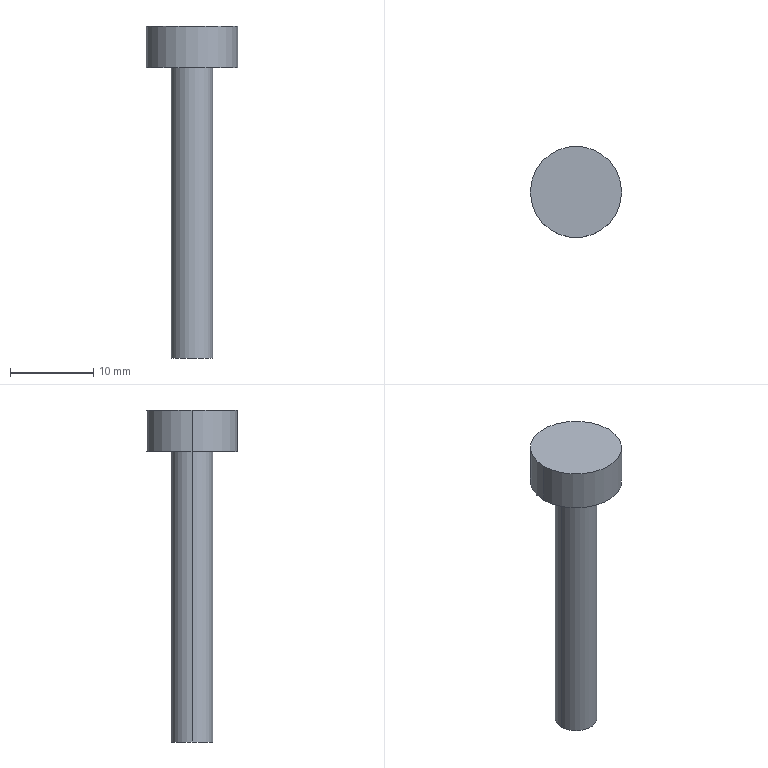Part | STEP file | Pull rod | 1 solid | 7 faces | box 11 x 11 x 40 mm | volume 1162 mm3 | cylinder 4 | plane 3 | commonest cylinder face diameters 5 x2 11 x2
STEP:
#1=CARTESIAN_POINT('',(0.,0.,0.));
#2=DIRECTION('',(0.,0.,1.));
#3=DIRECTION('',(1.,0.,0.));
#4=AXIS2_PLACEMENT_3D('',#1,#2,#3);
#5=CARTESIAN_POINT('',(-2.5,0.,-35.));
#6=VERTEX_POINT('',#5);
#7=CARTESIAN_POINT('',(2.5,0.,-35.));
#8=VERTEX_POINT('',#7);
#9=CARTESIAN_POINT('',(0.,0.,-35.));
#10=DIRECTION('',(0.,0.,-1.));
#11=DIRECTION('',(-1.,0.,0.));
#12=AXIS2_PLACEMENT_3D('',#9,#10,#11);
#13=CIRCLE('',#12,2.5);
#14=CARTESIAN_POINT('',(0.,0.,-35.));
#15=DIRECTION('',(0.,0.,1.));
#16=DIRECTION('',(1.,0.,0.));
#17=AXIS2_PLACEMENT_3D('',#14,#15,#16);
#18=CYLINDRICAL_SURFACE('',#17,2.5);
#19=CARTESIAN_POINT('',(3.142,0.));
#20=DIRECTION('',(-1.,0.));
#21=VECTOR('',#20,1.);
#22=LINE('',#19,#21);
#23=(GEOMETRIC_REPRESENTATION_CONTEXT(2)PARAMETRIC_REPRESENTATION_CONTEXT()REPRESENTATION_CONTEXT('',''));
#24=DEFINITIONAL_REPRESENTATION('',(#22),#23);
#25=PCURVE('',#18,#24);
#26=CARTESIAN_POINT('',(0.,0.,-35.));
#27=DIRECTION('',(0.,0.,-1.));
#28=DIRECTION('',(-1.,0.,0.));
#29=AXIS2_PLACEMENT_3D('',#26,#27,#28);
#30=PLANE('',#29);
#31=CARTESIAN_POINT('',(0.,0.));
#32=DIRECTION('',(1.,0.));
#33=AXIS2_PLACEMENT_2D('',#31,#32);
#34=CIRCLE('',#33,2.5);
#35=(GEOMETRIC_REPRESENTATION_CONTEXT(2)PARAMETRIC_REPRESENTATION_CONTEXT()REPRESENTATION_CONTEXT('',''));
#36=DEFINITIONAL_REPRESENTATION('',(#34),#35);
#37=PCURVE('',#30,#36);
#38=SURFACE_CURVE('',#13,(#25,#37),.PCURVE_S1.);
#39=EDGE_CURVE('',#6,#8,#38,.T.);
#40=ORIENTED_EDGE('',*,*,#39,.F.);
#41=CARTESIAN_POINT('',(-2.5,0.,0.));
#42=VERTEX_POINT('',#41);
#43=CARTESIAN_POINT('',(-2.5,0.,-35.));
#44=DIRECTION('',(0.,0.,1.));
#45=VECTOR('',#44,1.);
#46=LINE('',#43,#45);
#47=CARTESIAN_POINT('',(3.142,0.));
#48=DIRECTION('',(0.,1.));
#49=VECTOR('',#48,1.);
#50=LINE('',#47,#49);
#51=(GEOMETRIC_REPRESENTATION_CONTEXT(2)PARAMETRIC_REPRESENTATION_CONTEXT()REPRESENTATION_CONTEXT('',''));
#52=DEFINITIONAL_REPRESENTATION('',(#50),#51);
#53=PCURVE('',#18,#52);
#54=CARTESIAN_POINT('',(0.,0.,-35.));
#55=DIRECTION('',(0.,0.,1.));
#56=DIRECTION('',(1.,0.,0.));
#57=AXIS2_PLACEMENT_3D('',#54,#55,#56);
#58=CYLINDRICAL_SURFACE('',#57,2.5);
#59=CARTESIAN_POINT('',(3.142,0.));
#60=DIRECTION('',(0.,1.));
#61=VECTOR('',#60,1.);
#62=LINE('',#59,#61);
#63=(GEOMETRIC_REPRESENTATION_CONTEXT(2)PARAMETRIC_REPRESENTATION_CONTEXT()REPRESENTATION_CONTEXT('',''));
#64=DEFINITIONAL_REPRESENTATION('',(#62),#63);
#65=PCURVE('',#58,#64);
#66=SURFACE_CURVE('',#46,(#53,#65),.PCURVE_S1.);
#67=EDGE_CURVE('',#6,#42,#66,.T.);
#68=ORIENTED_EDGE('',*,*,#67,.T.);
#69=CARTESIAN_POINT('',(2.5,0.,0.));
#70=VERTEX_POINT('',#69);
#71=CARTESIAN_POINT('',(0.,0.,0.));
#72=DIRECTION('',(0.,0.,-1.));
#73=DIRECTION('',(1.,0.,0.));
#74=AXIS2_PLACEMENT_3D('',#71,#72,#73);
#75=CIRCLE('',#74,2.5);
#76=CARTESIAN_POINT('',(6.283,35.));
#77=DIRECTION('',(-1.,0.));
#78=VECTOR('',#77,1.);
#79=LINE('',#76,#78);
#80=(GEOMETRIC_REPRESENTATION_CONTEXT(2)PARAMETRIC_REPRESENTATION_CONTEXT()REPRESENTATION_CONTEXT('',''));
#81=DEFINITIONAL_REPRESENTATION('',(#79),#80);
#82=PCURVE('',#18,#81);
#83=CARTESIAN_POINT('',(0.,0.,0.));
#84=DIRECTION('',(0.,0.,1.));
#85=DIRECTION('',(1.,0.,0.));
#86=AXIS2_PLACEMENT_3D('',#83,#84,#85);
#87=PLANE('',#86);
#88=CARTESIAN_POINT('',(2.5,0.));
#89=CARTESIAN_POINT('',(2.5,-4.33));
#90=CARTESIAN_POINT('',(-1.25,-2.165));
#91=CARTESIAN_POINT('',(-5.,0.));
#92=CARTESIAN_POINT('',(-1.25,2.165));
#93=CARTESIAN_POINT('',(2.5,4.33));
#94=CARTESIAN_POINT('',(2.5,0.));
#95=(BOUNDED_CURVE()B_SPLINE_CURVE(2,(#88,#89,#90,#91,#92,#93,#94),.UNSPECIFIED.,.T.,.F.)B_SPLINE_CURVE_WITH_KNOTS((1,2,2,2,2,1),(-2.094,0.,2.094,4.189,6.283,8.378),.UNSPECIFIED.)CURVE()GEOMETRIC_REPRESENTATION_ITEM()RATIONAL_B_SPLINE_CURVE((1.,0.5,1.,0.5,1.,0.5,1.))REPRESENTATION_ITEM(''));
#96=(GEOMETRIC_REPRESENTATION_CONTEXT(2)PARAMETRIC_REPRESENTATION_CONTEXT()REPRESENTATION_CONTEXT('',''));
#97=DEFINITIONAL_REPRESENTATION('',(#95),#96);
#98=PCURVE('',#87,#97);
#99=SURFACE_CURVE('',#75,(#82,#98),.PCURVE_S1.);
#100=EDGE_CURVE('',#42,#70,#99,.T.);
#101=ORIENTED_EDGE('',*,*,#100,.T.);
#102=CARTESIAN_POINT('',(2.5,0.,-35.));
#103=DIRECTION('',(0.,0.,1.));
#104=VECTOR('',#103,1.);
#105=LINE('',#102,#104);
#106=CARTESIAN_POINT('',(0.,0.));
#107=DIRECTION('',(0.,1.));
#108=VECTOR('',#107,1.);
#109=LINE('',#106,#108);
#110=(GEOMETRIC_REPRESENTATION_CONTEXT(2)PARAMETRIC_REPRESENTATION_CONTEXT()REPRESENTATION_CONTEXT('',''));
#111=DEFINITIONAL_REPRESENTATION('',(#109),#110);
#112=PCURVE('',#18,#111);
#113=CARTESIAN_POINT('',(6.283,0.));
#114=DIRECTION('',(0.,1.));
#115=VECTOR('',#114,1.);
#116=LINE('',#113,#115);
#117=(GEOMETRIC_REPRESENTATION_CONTEXT(2)PARAMETRIC_REPRESENTATION_CONTEXT()REPRESENTATION_CONTEXT('',''));
#118=DEFINITIONAL_REPRESENTATION('',(#116),#117);
#119=PCURVE('',#58,#118);
#120=SURFACE_CURVE('',#105,(#112,#119),.PCURVE_S1.);
#121=EDGE_CURVE('',#8,#70,#120,.T.);
#122=ORIENTED_EDGE('',*,*,#121,.F.);
#123=EDGE_LOOP('',(#40,#68,#101,#122));
#124=FACE_BOUND('',#123,.T.);
#125=ADVANCED_FACE('',(#124),#18,.T.);
#126=CARTESIAN_POINT('',(5.5,0.,5.));
#127=VERTEX_POINT('',#126);
#128=CARTESIAN_POINT('',(-5.5,0.,5.));
#129=VERTEX_POINT('',#128);
#130=CARTESIAN_POINT('',(0.,0.,5.));
#131=DIRECTION('',(0.,0.,1.));
#132=DIRECTION('',(1.,0.,0.));
#133=AXIS2_PLACEMENT_3D('',#130,#131,#132);
#134=CIRCLE('',#133,5.5);
#135=CARTESIAN_POINT('',(0.,0.,5.));
#136=DIRECTION('',(0.,0.,-1.));
#137=DIRECTION('',(-1.,0.,0.));
#138=AXIS2_PLACEMENT_3D('',#135,#136,#137);
#139=CYLINDRICAL_SURFACE('',#138,5.5);
#140=CARTESIAN_POINT('',(3.142,0.));
#141=DIRECTION('',(-1.,0.));
#142=VECTOR('',#141,1.);
#143=LINE('',#140,#142);
#144=(GEOMETRIC_REPRESENTATION_CONTEXT(2)PARAMETRIC_REPRESENTATION_CONTEXT()REPRESENTATION_CONTEXT('',''));
#145=DEFINITIONAL_REPRESENTATION('',(#143),#144);
#146=PCURVE('',#139,#145);
#147=CARTESIAN_POINT('',(0.,0.,5.));
#148=DIRECTION('',(0.,0.,1.));
#149=DIRECTION('',(1.,0.,0.));
#150=AXIS2_PLACEMENT_3D('',#147,#148,#149);
#151=PLANE('',#150);
#152=CARTESIAN_POINT('',(0.,0.));
#153=DIRECTION('',(1.,0.));
#154=AXIS2_PLACEMENT_2D('',#152,#153);
#155=CIRCLE('',#154,5.5);
#156=(GEOMETRIC_REPRESENTATION_CONTEXT(2)PARAMETRIC_REPRESENTATION_CONTEXT()REPRESENTATION_CONTEXT('',''));
#157=DEFINITIONAL_REPRESENTATION('',(#155),#156);
#158=PCURVE('',#151,#157);
#159=SURFACE_CURVE('',#134,(#146,#158),.PCURVE_S1.);
#160=EDGE_CURVE('',#127,#129,#159,.T.);
#161=ORIENTED_EDGE('',*,*,#160,.F.);
#162=CARTESIAN_POINT('',(5.5,0.,0.));
#163=VERTEX_POINT('',#162);
#164=CARTESIAN_POINT('',(5.5,0.,5.));
#165=DIRECTION('',(0.,0.,-1.));
#166=VECTOR('',#165,1.);
#167=LINE('',#164,#166);
#168=CARTESIAN_POINT('',(3.142,0.));
#169=DIRECTION('',(0.,1.));
#170=VECTOR('',#169,1.);
#171=LINE('',#168,#170);
#172=(GEOMETRIC_REPRESENTATION_CONTEXT(2)PARAMETRIC_REPRESENTATION_CONTEXT()REPRESENTATION_CONTEXT('',''));
#173=DEFINITIONAL_REPRESENTATION('',(#171),#172);
#174=PCURVE('',#139,#173);
#175=CARTESIAN_POINT('',(0.,0.,5.));
#176=DIRECTION('',(0.,0.,-1.));
#177=DIRECTION('',(-1.,0.,0.));
#178=AXIS2_PLACEMENT_3D('',#175,#176,#177);
#179=CYLINDRICAL_SURFACE('',#178,5.5);
#180=CARTESIAN_POINT('',(3.142,0.));
#181=DIRECTION('',(0.,1.));
#182=VECTOR('',#181,1.);
#183=LINE('',#180,#182);
#184=(GEOMETRIC_REPRESENTATION_CONTEXT(2)PARAMETRIC_REPRESENTATION_CONTEXT()REPRESENTATION_CONTEXT('',''));
#185=DEFINITIONAL_REPRESENTATION('',(#183),#184);
#186=PCURVE('',#179,#185);
#187=SURFACE_CURVE('',#167,(#174,#186),.PCURVE_S1.);
#188=EDGE_CURVE('',#127,#163,#187,.T.);
#189=ORIENTED_EDGE('',*,*,#188,.T.);
#190=CARTESIAN_POINT('',(-5.5,0.,0.));
#191=VERTEX_POINT('',#190);
#192=CARTESIAN_POINT('',(0.,0.,0.));
#193=DIRECTION('',(0.,0.,1.));
#194=DIRECTION('',(1.,0.,0.));
#195=AXIS2_PLACEMENT_3D('',#192,#193,#194);
#196=CIRCLE('',#195,5.5);
#197=CARTESIAN_POINT('',(3.142,5.));
#198=DIRECTION('',(-1.,0.));
#199=VECTOR('',#198,1.);
#200=LINE('',#197,#199);
#201=(GEOMETRIC_REPRESENTATION_CONTEXT(2)PARAMETRIC_REPRESENTATION_CONTEXT()REPRESENTATION_CONTEXT('',''));
#202=DEFINITIONAL_REPRESENTATION('',(#200),#201);
#203=PCURVE('',#139,#202);
#204=CARTESIAN_POINT('',(0.,0.));
#205=DIRECTION('',(1.,0.));
#206=AXIS2_PLACEMENT_2D('',#204,#205);
#207=CIRCLE('',#206,5.5);
#208=(GEOMETRIC_REPRESENTATION_CONTEXT(2)PARAMETRIC_REPRESENTATION_CONTEXT()REPRESENTATION_CONTEXT('',''));
#209=DEFINITIONAL_REPRESENTATION('',(#207),#208);
#210=PCURVE('',#87,#209);
#211=SURFACE_CURVE('',#196,(#203,#210),.PCURVE_S1.);
#212=EDGE_CURVE('',#163,#191,#211,.T.);
#213=ORIENTED_EDGE('',*,*,#212,.T.);
#214=CARTESIAN_POINT('',(-5.5,0.,5.));
#215=DIRECTION('',(0.,0.,-1.));
#216=VECTOR('',#215,1.);
#217=LINE('',#214,#216);
#218=CARTESIAN_POINT('',(0.,0.));
#219=DIRECTION('',(0.,1.));
#220=VECTOR('',#219,1.);
#221=LINE('',#218,#220);
#222=(GEOMETRIC_REPRESENTATION_CONTEXT(2)PARAMETRIC_REPRESENTATION_CONTEXT()REPRESENTATION_CONTEXT('',''));
#223=DEFINITIONAL_REPRESENTATION('',(#221),#222);
#224=PCURVE('',#139,#223);
#225=CARTESIAN_POINT('',(6.283,0.));
#226=DIRECTION('',(0.,1.));
#227=VECTOR('',#226,1.);
#228=LINE('',#225,#227);
#229=(GEOMETRIC_REPRESENTATION_CONTEXT(2)PARAMETRIC_REPRESENTATION_CONTEXT()REPRESENTATION_CONTEXT('',''));
#230=DEFINITIONAL_REPRESENTATION('',(#228),#229);
#231=PCURVE('',#179,#230);
#232=SURFACE_CURVE('',#217,(#224,#231),.PCURVE_S1.);
#233=EDGE_CURVE('',#129,#191,#232,.T.);
#234=ORIENTED_EDGE('',*,*,#233,.F.);
#235=EDGE_LOOP('',(#161,#189,#213,#234));
#236=FACE_BOUND('',#235,.T.);
#237=ADVANCED_FACE('',(#236),#139,.T.);
#238=CARTESIAN_POINT('',(0.,0.,0.));
#239=DIRECTION('',(0.,0.,1.));
#240=DIRECTION('',(1.,0.,0.));
#241=AXIS2_PLACEMENT_3D('',#238,#239,#240);
#242=CIRCLE('',#241,5.5);
#243=CARTESIAN_POINT('',(0.,0.));
#244=DIRECTION('',(1.,0.));
#245=AXIS2_PLACEMENT_2D('',#243,#244);
#246=CIRCLE('',#245,5.5);
#247=(GEOMETRIC_REPRESENTATION_CONTEXT(2)PARAMETRIC_REPRESENTATION_CONTEXT()REPRESENTATION_CONTEXT('',''));
#248=DEFINITIONAL_REPRESENTATION('',(#246),#247);
#249=PCURVE('',#87,#248);
#250=CARTESIAN_POINT('',(9.425,5.));
#251=DIRECTION('',(-1.,0.));
#252=VECTOR('',#251,1.);
#253=LINE('',#250,#252);
#254=(GEOMETRIC_REPRESENTATION_CONTEXT(2)PARAMETRIC_REPRESENTATION_CONTEXT()REPRESENTATION_CONTEXT('',''));
#255=DEFINITIONAL_REPRESENTATION('',(#253),#254);
#256=PCURVE('',#179,#255);
#257=SURFACE_CURVE('',#242,(#249,#256),.PCURVE_S1.);
#258=EDGE_CURVE('',#191,#163,#257,.T.);
#259=ORIENTED_EDGE('',*,*,#258,.F.);
#260=ORIENTED_EDGE('',*,*,#212,.F.);
#261=EDGE_LOOP('',(#259,#260));
#262=FACE_BOUND('',#261,.T.);
#263=CARTESIAN_POINT('',(0.,0.,0.));
#264=DIRECTION('',(0.,0.,-1.));
#265=DIRECTION('',(1.,0.,0.));
#266=AXIS2_PLACEMENT_3D('',#263,#264,#265);
#267=CIRCLE('',#266,2.5);
#268=CARTESIAN_POINT('',(2.5,0.));
#269=CARTESIAN_POINT('',(2.5,-4.33));
#270=CARTESIAN_POINT('',(-1.25,-2.165));
#271=CARTESIAN_POINT('',(-5.,0.));
#272=CARTESIAN_POINT('',(-1.25,2.165));
#273=CARTESIAN_POINT('',(2.5,4.33));
#274=CARTESIAN_POINT('',(2.5,0.));
#275=(BOUNDED_CURVE()B_SPLINE_CURVE(2,(#268,#269,#270,#271,#272,#273,#274),.UNSPECIFIED.,.T.,.F.)B_SPLINE_CURVE_WITH_KNOTS((1,2,2,2,2,1),(-2.094,0.,2.094,4.189,6.283,8.378),.UNSPECIFIED.)CURVE()GEOMETRIC_REPRESENTATION_ITEM()RATIONAL_B_SPLINE_CURVE((1.,0.5,1.,0.5,1.,0.5,1.))REPRESENTATION_ITEM(''));
#276=(GEOMETRIC_REPRESENTATION_CONTEXT(2)PARAMETRIC_REPRESENTATION_CONTEXT()REPRESENTATION_CONTEXT('',''));
#277=DEFINITIONAL_REPRESENTATION('',(#275),#276);
#278=PCURVE('',#87,#277);
#279=CARTESIAN_POINT('',(6.283,35.));
#280=DIRECTION('',(-1.,0.));
#281=VECTOR('',#280,1.);
#282=LINE('',#279,#281);
#283=(GEOMETRIC_REPRESENTATION_CONTEXT(2)PARAMETRIC_REPRESENTATION_CONTEXT()REPRESENTATION_CONTEXT('',''));
#284=DEFINITIONAL_REPRESENTATION('',(#282),#283);
#285=PCURVE('',#58,#284);
#286=SURFACE_CURVE('',#267,(#278,#285),.PCURVE_S1.);
#287=EDGE_CURVE('',#70,#42,#286,.T.);
#288=ORIENTED_EDGE('',*,*,#287,.F.);
#289=ORIENTED_EDGE('',*,*,#100,.F.);
#290=EDGE_LOOP('',(#288,#289));
#291=FACE_BOUND('',#290,.T.);
#292=ADVANCED_FACE('',(#262,#291),#87,.F.);
#293=ORIENTED_EDGE('',*,*,#188,.F.);
#294=CARTESIAN_POINT('',(0.,0.,5.));
#295=DIRECTION('',(0.,0.,1.));
#296=DIRECTION('',(1.,0.,0.));
#297=AXIS2_PLACEMENT_3D('',#294,#295,#296);
#298=CIRCLE('',#297,5.5);
#299=CARTESIAN_POINT('',(9.425,0.));
#300=DIRECTION('',(-1.,0.));
#301=VECTOR('',#300,1.);
#302=LINE('',#299,#301);
#303=(GEOMETRIC_REPRESENTATION_CONTEXT(2)PARAMETRIC_REPRESENTATION_CONTEXT()REPRESENTATION_CONTEXT('',''));
#304=DEFINITIONAL_REPRESENTATION('',(#302),#303);
#305=PCURVE('',#179,#304);
#306=CARTESIAN_POINT('',(0.,0.));
#307=DIRECTION('',(1.,0.));
#308=AXIS2_PLACEMENT_2D('',#306,#307);
#309=CIRCLE('',#308,5.5);
#310=(GEOMETRIC_REPRESENTATION_CONTEXT(2)PARAMETRIC_REPRESENTATION_CONTEXT()REPRESENTATION_CONTEXT('',''));
#311=DEFINITIONAL_REPRESENTATION('',(#309),#310);
#312=PCURVE('',#151,#311);
#313=SURFACE_CURVE('',#298,(#305,#312),.PCURVE_S1.);
#314=EDGE_CURVE('',#129,#127,#313,.T.);
#315=ORIENTED_EDGE('',*,*,#314,.F.);
#316=ORIENTED_EDGE('',*,*,#233,.T.);
#317=ORIENTED_EDGE('',*,*,#258,.T.);
#318=EDGE_LOOP('',(#293,#315,#316,#317));
#319=FACE_BOUND('',#318,.T.);
#320=ADVANCED_FACE('',(#319),#179,.T.);
#321=ORIENTED_EDGE('',*,*,#314,.T.);
#322=ORIENTED_EDGE('',*,*,#160,.T.);
#323=EDGE_LOOP('',(#321,#322));
#324=FACE_BOUND('',#323,.T.);
#325=ADVANCED_FACE('',(#324),#151,.T.);
#326=ORIENTED_EDGE('',*,*,#67,.F.);
#327=CARTESIAN_POINT('',(0.,0.,-35.));
#328=DIRECTION('',(0.,0.,-1.));
#329=DIRECTION('',(-1.,0.,0.));
#330=AXIS2_PLACEMENT_3D('',#327,#328,#329);
#331=CIRCLE('',#330,2.5);
#332=CARTESIAN_POINT('',(9.425,0.));
#333=DIRECTION('',(-1.,0.));
#334=VECTOR('',#333,1.);
#335=LINE('',#332,#334);
#336=(GEOMETRIC_REPRESENTATION_CONTEXT(2)PARAMETRIC_REPRESENTATION_CONTEXT()REPRESENTATION_CONTEXT('',''));
#337=DEFINITIONAL_REPRESENTATION('',(#335),#336);
#338=PCURVE('',#58,#337);
#339=CARTESIAN_POINT('',(0.,0.));
#340=DIRECTION('',(1.,0.));
#341=AXIS2_PLACEMENT_2D('',#339,#340);
#342=CIRCLE('',#341,2.5);
#343=(GEOMETRIC_REPRESENTATION_CONTEXT(2)PARAMETRIC_REPRESENTATION_CONTEXT()REPRESENTATION_CONTEXT('',''));
#344=DEFINITIONAL_REPRESENTATION('',(#342),#343);
#345=PCURVE('',#30,#344);
#346=SURFACE_CURVE('',#331,(#338,#345),.PCURVE_S1.);
#347=EDGE_CURVE('',#8,#6,#346,.T.);
#348=ORIENTED_EDGE('',*,*,#347,.F.);
#349=ORIENTED_EDGE('',*,*,#121,.T.);
#350=ORIENTED_EDGE('',*,*,#287,.T.);
#351=EDGE_LOOP('',(#326,#348,#349,#350));
#352=FACE_BOUND('',#351,.T.);
#353=ADVANCED_FACE('',(#352),#58,.T.);
#354=ORIENTED_EDGE('',*,*,#347,.T.);
#355=ORIENTED_EDGE('',*,*,#39,.T.);
#356=EDGE_LOOP('',(#354,#355));
#357=FACE_BOUND('',#356,.T.);
#358=ADVANCED_FACE('',(#357),#30,.T.);
#359=CLOSED_SHELL('',(#125,#237,#292,#320,#325,#353,#358));
#360=MANIFOLD_SOLID_BREP('',#359);
#361=(LENGTH_UNIT()NAMED_UNIT(*)SI_UNIT(.MILLI.,.METRE.));
#362=UNCERTAINTY_MEASURE_WITH_UNIT(LENGTH_MEASURE(0.0000001),#361,'','');
#363=(NAMED_UNIT(*)PLANE_ANGLE_UNIT()SI_UNIT($,.RADIAN.));
#364=(NAMED_UNIT(*)SI_UNIT($,.STERADIAN.)SOLID_ANGLE_UNIT());
#365=(GEOMETRIC_REPRESENTATION_CONTEXT(3)GLOBAL_UNCERTAINTY_ASSIGNED_CONTEXT((#362))GLOBAL_UNIT_ASSIGNED_CONTEXT((#361,#363,#364))REPRESENTATION_CONTEXT('',''));
#366=ADVANCED_BREP_SHAPE_REPRESENTATION('',(#4,#360),#365);